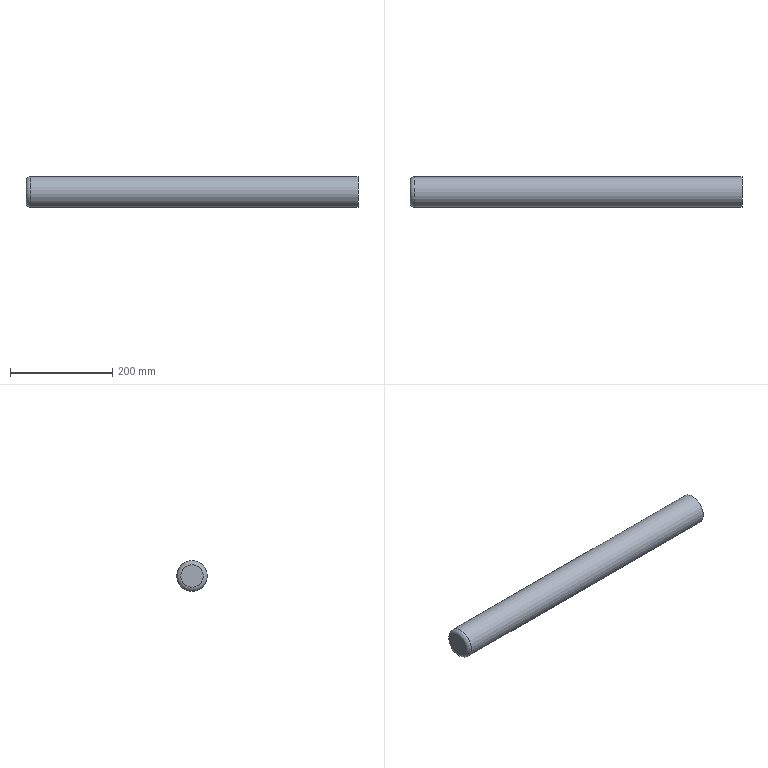Part | STEP file | solid 161 | 1 solid | 4 faces | box 650 x 60 x 60 mm | volume 1835397 mm3 | plane 2 | cylinder 1 | torus 1 | commonest cylinder face diameters 60 x1